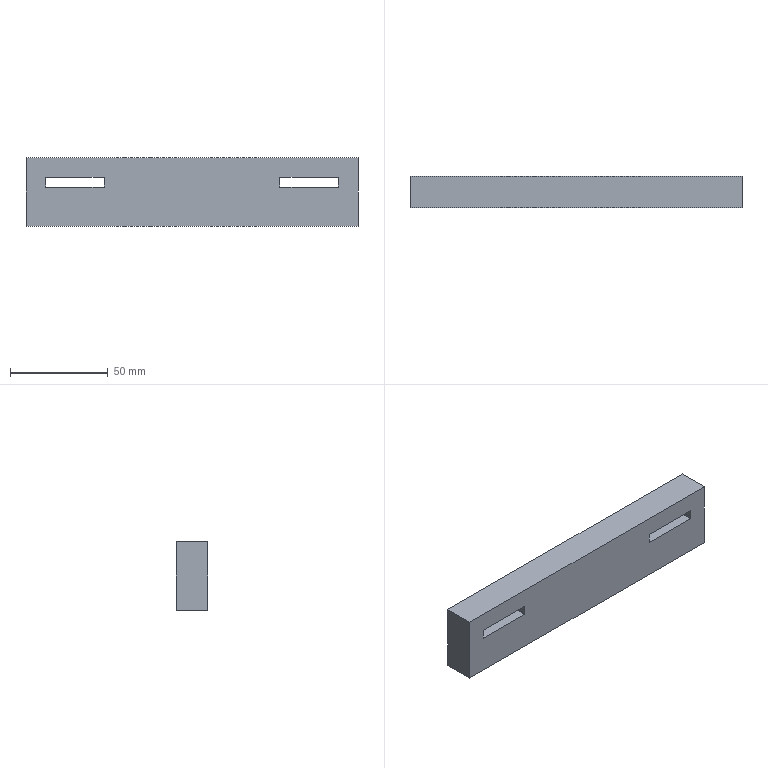Part | STEP file | Tube necking machine_id730_x_t | 1 solid | 14 faces | box 170 x 16 x 35 mm | volume 90400 mm3 | plane 14
STEP:
#1=CARTESIAN_POINT('',(0.,0.,0.));
#2=DIRECTION('',(0.,0.,1.));
#3=DIRECTION('',(1.,0.,0.));
#4=AXIS2_PLACEMENT_3D('',#1,#2,#3);
#5=CARTESIAN_POINT('',(-75.,-243.,191.));
#6=VERTEX_POINT('',#5);
#7=CARTESIAN_POINT('',(-75.,-243.,196.));
#8=VERTEX_POINT('',#7);
#9=CARTESIAN_POINT('',(-75.,-243.,191.));
#10=DIRECTION('',(0.,0.,1.));
#11=VECTOR('',#10,1.);
#12=LINE('',#9,#11);
#13=CARTESIAN_POINT('',(0.,-243.,0.));
#14=DIRECTION('',(0.,-1.,0.));
#15=DIRECTION('',(0.,0.,-1.));
#16=AXIS2_PLACEMENT_3D('',#13,#14,#15);
#17=PLANE('',#16);
#18=CARTESIAN_POINT('',(-191.,-75.));
#19=DIRECTION('',(-1.,0.));
#20=VECTOR('',#19,1.);
#21=LINE('',#18,#20);
#22=(GEOMETRIC_REPRESENTATION_CONTEXT(2)PARAMETRIC_REPRESENTATION_CONTEXT()REPRESENTATION_CONTEXT('',''));
#23=DEFINITIONAL_REPRESENTATION('',(#21),#22);
#24=PCURVE('',#17,#23);
#25=CARTESIAN_POINT('',(-75.,-243.,191.));
#26=DIRECTION('',(1.,0.,0.));
#27=DIRECTION('',(0.,0.,-1.));
#28=AXIS2_PLACEMENT_3D('',#25,#26,#27);
#29=PLANE('',#28);
#30=CARTESIAN_POINT('',(0.,0.));
#31=DIRECTION('',(-1.,0.));
#32=VECTOR('',#31,1.);
#33=LINE('',#30,#32);
#34=(GEOMETRIC_REPRESENTATION_CONTEXT(2)PARAMETRIC_REPRESENTATION_CONTEXT()REPRESENTATION_CONTEXT('',''));
#35=DEFINITIONAL_REPRESENTATION('',(#33),#34);
#36=PCURVE('',#29,#35);
#37=SURFACE_CURVE('',#12,(#24,#36),.PCURVE_S1.);
#38=EDGE_CURVE('',#6,#8,#37,.T.);
#39=ORIENTED_EDGE('',*,*,#38,.F.);
#40=CARTESIAN_POINT('',(-45.,-243.,191.));
#41=VERTEX_POINT('',#40);
#42=CARTESIAN_POINT('',(-40.,-243.,191.));
#43=DIRECTION('',(-1.,0.,0.));
#44=VECTOR('',#43,1.);
#45=LINE('',#42,#44);
#46=CARTESIAN_POINT('',(-191.,-40.));
#47=DIRECTION('',(0.,-1.));
#48=VECTOR('',#47,1.);
#49=LINE('',#46,#48);
#50=(GEOMETRIC_REPRESENTATION_CONTEXT(2)PARAMETRIC_REPRESENTATION_CONTEXT()REPRESENTATION_CONTEXT('',''));
#51=DEFINITIONAL_REPRESENTATION('',(#49),#50);
#52=PCURVE('',#17,#51);
#53=CARTESIAN_POINT('',(-40.,-243.,191.));
#54=DIRECTION('',(0.,0.,1.));
#55=DIRECTION('',(1.,0.,0.));
#56=AXIS2_PLACEMENT_3D('',#53,#54,#55);
#57=PLANE('',#56);
#58=CARTESIAN_POINT('',(0.,0.));
#59=DIRECTION('',(-1.,0.));
#60=VECTOR('',#59,1.);
#61=LINE('',#58,#60);
#62=(GEOMETRIC_REPRESENTATION_CONTEXT(2)PARAMETRIC_REPRESENTATION_CONTEXT()REPRESENTATION_CONTEXT('',''));
#63=DEFINITIONAL_REPRESENTATION('',(#61),#62);
#64=PCURVE('',#57,#63);
#65=SURFACE_CURVE('',#45,(#52,#64),.PCURVE_S1.);
#66=EDGE_CURVE('',#41,#6,#65,.T.);
#67=ORIENTED_EDGE('',*,*,#66,.F.);
#68=CARTESIAN_POINT('',(-45.,-243.,196.));
#69=VERTEX_POINT('',#68);
#70=CARTESIAN_POINT('',(-45.,-243.,0.));
#71=DIRECTION('',(0.,0.,-1.));
#72=VECTOR('',#71,1.);
#73=LINE('',#70,#72);
#74=CARTESIAN_POINT('',(0.,-45.));
#75=DIRECTION('',(1.,0.));
#76=VECTOR('',#75,1.);
#77=LINE('',#74,#76);
#78=(GEOMETRIC_REPRESENTATION_CONTEXT(2)PARAMETRIC_REPRESENTATION_CONTEXT()REPRESENTATION_CONTEXT('',''));
#79=DEFINITIONAL_REPRESENTATION('',(#77),#78);
#80=PCURVE('',#17,#79);
#81=CARTESIAN_POINT('',(-45.,-243.,196.));
#82=DIRECTION('',(-1.,0.,0.));
#83=DIRECTION('',(0.,0.,1.));
#84=AXIS2_PLACEMENT_3D('',#81,#82,#83);
#85=PLANE('',#84);
#86=CARTESIAN_POINT('',(-196.,0.));
#87=DIRECTION('',(-1.,0.));
#88=VECTOR('',#87,1.);
#89=LINE('',#86,#88);
#90=(GEOMETRIC_REPRESENTATION_CONTEXT(2)PARAMETRIC_REPRESENTATION_CONTEXT()REPRESENTATION_CONTEXT('',''));
#91=DEFINITIONAL_REPRESENTATION('',(#89),#90);
#92=PCURVE('',#85,#91);
#93=SURFACE_CURVE('',#73,(#80,#92),.PCURVE_S1.);
#94=EDGE_CURVE('',#69,#41,#93,.T.);
#95=ORIENTED_EDGE('',*,*,#94,.F.);
#96=CARTESIAN_POINT('',(-75.,-243.,196.));
#97=DIRECTION('',(1.,0.,0.));
#98=VECTOR('',#97,1.);
#99=LINE('',#96,#98);
#100=CARTESIAN_POINT('',(-196.,-75.));
#101=DIRECTION('',(0.,1.));
#102=VECTOR('',#101,1.);
#103=LINE('',#100,#102);
#104=(GEOMETRIC_REPRESENTATION_CONTEXT(2)PARAMETRIC_REPRESENTATION_CONTEXT()REPRESENTATION_CONTEXT('',''));
#105=DEFINITIONAL_REPRESENTATION('',(#103),#104);
#106=PCURVE('',#17,#105);
#107=CARTESIAN_POINT('',(-75.,-243.,196.));
#108=DIRECTION('',(0.,0.,-1.));
#109=DIRECTION('',(-1.,0.,0.));
#110=AXIS2_PLACEMENT_3D('',#107,#108,#109);
#111=PLANE('',#110);
#112=CARTESIAN_POINT('',(0.,0.));
#113=DIRECTION('',(-1.,0.));
#114=VECTOR('',#113,1.);
#115=LINE('',#112,#114);
#116=(GEOMETRIC_REPRESENTATION_CONTEXT(2)PARAMETRIC_REPRESENTATION_CONTEXT()REPRESENTATION_CONTEXT('',''));
#117=DEFINITIONAL_REPRESENTATION('',(#115),#116);
#118=PCURVE('',#111,#117);
#119=SURFACE_CURVE('',#99,(#106,#118),.PCURVE_S1.);
#120=EDGE_CURVE('',#8,#69,#119,.T.);
#121=ORIENTED_EDGE('',*,*,#120,.F.);
#122=EDGE_LOOP('',(#39,#67,#95,#121));
#123=FACE_BOUND('',#122,.T.);
#124=CARTESIAN_POINT('',(-85.,-243.,206.));
#125=VERTEX_POINT('',#124);
#126=CARTESIAN_POINT('',(-85.,-243.,171.));
#127=VERTEX_POINT('',#126);
#128=CARTESIAN_POINT('',(-85.,-243.,206.));
#129=DIRECTION('',(0.,0.,-1.));
#130=VECTOR('',#129,1.);
#131=LINE('',#128,#130);
#132=CARTESIAN_POINT('',(-206.,-85.));
#133=DIRECTION('',(1.,0.));
#134=VECTOR('',#133,1.);
#135=LINE('',#132,#134);
#136=(GEOMETRIC_REPRESENTATION_CONTEXT(2)PARAMETRIC_REPRESENTATION_CONTEXT()REPRESENTATION_CONTEXT('',''));
#137=DEFINITIONAL_REPRESENTATION('',(#135),#136);
#138=PCURVE('',#17,#137);
#139=CARTESIAN_POINT('',(-85.,-243.,206.));
#140=DIRECTION('',(-1.,0.,0.));
#141=DIRECTION('',(0.,0.,1.));
#142=AXIS2_PLACEMENT_3D('',#139,#140,#141);
#143=PLANE('',#142);
#144=CARTESIAN_POINT('',(0.,0.));
#145=DIRECTION('',(-1.,0.));
#146=VECTOR('',#145,1.);
#147=LINE('',#144,#146);
#148=(GEOMETRIC_REPRESENTATION_CONTEXT(2)PARAMETRIC_REPRESENTATION_CONTEXT()REPRESENTATION_CONTEXT('',''));
#149=DEFINITIONAL_REPRESENTATION('',(#147),#148);
#150=PCURVE('',#143,#149);
#151=SURFACE_CURVE('',#131,(#138,#150),.PCURVE_S1.);
#152=EDGE_CURVE('',#125,#127,#151,.T.);
#153=ORIENTED_EDGE('',*,*,#152,.F.);
#154=CARTESIAN_POINT('',(85.,-243.,206.));
#155=VERTEX_POINT('',#154);
#156=CARTESIAN_POINT('',(85.,-243.,206.));
#157=DIRECTION('',(-1.,0.,0.));
#158=VECTOR('',#157,1.);
#159=LINE('',#156,#158);
#160=CARTESIAN_POINT('',(-206.,85.));
#161=DIRECTION('',(0.,-1.));
#162=VECTOR('',#161,1.);
#163=LINE('',#160,#162);
#164=(GEOMETRIC_REPRESENTATION_CONTEXT(2)PARAMETRIC_REPRESENTATION_CONTEXT()REPRESENTATION_CONTEXT('',''));
#165=DEFINITIONAL_REPRESENTATION('',(#163),#164);
#166=PCURVE('',#17,#165);
#167=CARTESIAN_POINT('',(85.,-243.,206.));
#168=DIRECTION('',(0.,0.,1.));
#169=DIRECTION('',(1.,0.,0.));
#170=AXIS2_PLACEMENT_3D('',#167,#168,#169);
#171=PLANE('',#170);
#172=CARTESIAN_POINT('',(0.,0.));
#173=DIRECTION('',(-1.,0.));
#174=VECTOR('',#173,1.);
#175=LINE('',#172,#174);
#176=(GEOMETRIC_REPRESENTATION_CONTEXT(2)PARAMETRIC_REPRESENTATION_CONTEXT()REPRESENTATION_CONTEXT('',''));
#177=DEFINITIONAL_REPRESENTATION('',(#175),#176);
#178=PCURVE('',#171,#177);
#179=SURFACE_CURVE('',#159,(#166,#178),.PCURVE_S1.);
#180=EDGE_CURVE('',#155,#125,#179,.T.);
#181=ORIENTED_EDGE('',*,*,#180,.F.);
#182=CARTESIAN_POINT('',(85.,-243.,171.));
#183=VERTEX_POINT('',#182);
#184=CARTESIAN_POINT('',(85.,-243.,171.));
#185=DIRECTION('',(0.,0.,1.));
#186=VECTOR('',#185,1.);
#187=LINE('',#184,#186);
#188=CARTESIAN_POINT('',(-171.,85.));
#189=DIRECTION('',(-1.,0.));
#190=VECTOR('',#189,1.);
#191=LINE('',#188,#190);
#192=(GEOMETRIC_REPRESENTATION_CONTEXT(2)PARAMETRIC_REPRESENTATION_CONTEXT()REPRESENTATION_CONTEXT('',''));
#193=DEFINITIONAL_REPRESENTATION('',(#191),#192);
#194=PCURVE('',#17,#193);
#195=CARTESIAN_POINT('',(85.,-243.,171.));
#196=DIRECTION('',(1.,0.,0.));
#197=DIRECTION('',(0.,0.,-1.));
#198=AXIS2_PLACEMENT_3D('',#195,#196,#197);
#199=PLANE('',#198);
#200=CARTESIAN_POINT('',(0.,0.));
#201=DIRECTION('',(-1.,0.));
#202=VECTOR('',#201,1.);
#203=LINE('',#200,#202);
#204=(GEOMETRIC_REPRESENTATION_CONTEXT(2)PARAMETRIC_REPRESENTATION_CONTEXT()REPRESENTATION_CONTEXT('',''));
#205=DEFINITIONAL_REPRESENTATION('',(#203),#204);
#206=PCURVE('',#199,#205);
#207=SURFACE_CURVE('',#187,(#194,#206),.PCURVE_S1.);
#208=EDGE_CURVE('',#183,#155,#207,.T.);
#209=ORIENTED_EDGE('',*,*,#208,.F.);
#210=CARTESIAN_POINT('',(-85.,-243.,171.));
#211=DIRECTION('',(1.,0.,0.));
#212=VECTOR('',#211,1.);
#213=LINE('',#210,#212);
#214=CARTESIAN_POINT('',(-171.,-85.));
#215=DIRECTION('',(0.,1.));
#216=VECTOR('',#215,1.);
#217=LINE('',#214,#216);
#218=(GEOMETRIC_REPRESENTATION_CONTEXT(2)PARAMETRIC_REPRESENTATION_CONTEXT()REPRESENTATION_CONTEXT('',''));
#219=DEFINITIONAL_REPRESENTATION('',(#217),#218);
#220=PCURVE('',#17,#219);
#221=CARTESIAN_POINT('',(-85.,-243.,171.));
#222=DIRECTION('',(0.,0.,-1.));
#223=DIRECTION('',(-1.,0.,0.));
#224=AXIS2_PLACEMENT_3D('',#221,#222,#223);
#225=PLANE('',#224);
#226=CARTESIAN_POINT('',(0.,0.));
#227=DIRECTION('',(-1.,0.));
#228=VECTOR('',#227,1.);
#229=LINE('',#226,#228);
#230=(GEOMETRIC_REPRESENTATION_CONTEXT(2)PARAMETRIC_REPRESENTATION_CONTEXT()REPRESENTATION_CONTEXT('',''));
#231=DEFINITIONAL_REPRESENTATION('',(#229),#230);
#232=PCURVE('',#225,#231);
#233=SURFACE_CURVE('',#213,(#220,#232),.PCURVE_S1.);
#234=EDGE_CURVE('',#127,#183,#233,.T.);
#235=ORIENTED_EDGE('',*,*,#234,.F.);
#236=EDGE_LOOP('',(#153,#181,#209,#235));
#237=FACE_BOUND('',#236,.T.);
#238=CARTESIAN_POINT('',(45.,-243.,196.));
#239=VERTEX_POINT('',#238);
#240=CARTESIAN_POINT('',(75.,-243.,196.));
#241=VERTEX_POINT('',#240);
#242=CARTESIAN_POINT('',(0.,-243.,196.));
#243=DIRECTION('',(1.,0.,0.));
#244=VECTOR('',#243,1.);
#245=LINE('',#242,#244);
#246=CARTESIAN_POINT('',(-196.,0.));
#247=DIRECTION('',(0.,1.));
#248=VECTOR('',#247,1.);
#249=LINE('',#246,#248);
#250=(GEOMETRIC_REPRESENTATION_CONTEXT(2)PARAMETRIC_REPRESENTATION_CONTEXT()REPRESENTATION_CONTEXT('',''));
#251=DEFINITIONAL_REPRESENTATION('',(#249),#250);
#252=PCURVE('',#17,#251);
#253=CARTESIAN_POINT('',(40.,-259.,196.));
#254=DIRECTION('',(0.,0.,-1.));
#255=DIRECTION('',(1.,0.,0.));
#256=AXIS2_PLACEMENT_3D('',#253,#254,#255);
#257=PLANE('',#256);
#258=CARTESIAN_POINT('',(-40.,-16.));
#259=DIRECTION('',(1.,0.));
#260=VECTOR('',#259,1.);
#261=LINE('',#258,#260);
#262=(GEOMETRIC_REPRESENTATION_CONTEXT(2)PARAMETRIC_REPRESENTATION_CONTEXT()REPRESENTATION_CONTEXT('',''));
#263=DEFINITIONAL_REPRESENTATION('',(#261),#262);
#264=PCURVE('',#257,#263);
#265=SURFACE_CURVE('',#245,(#252,#264),.PCURVE_S1.);
#266=EDGE_CURVE('',#239,#241,#265,.T.);
#267=ORIENTED_EDGE('',*,*,#266,.F.);
#268=CARTESIAN_POINT('',(45.,-243.,191.));
#269=VERTEX_POINT('',#268);
#270=CARTESIAN_POINT('',(45.,-243.,0.));
#271=DIRECTION('',(0.,0.,1.));
#272=VECTOR('',#271,1.);
#273=LINE('',#270,#272);
#274=CARTESIAN_POINT('',(0.,45.));
#275=DIRECTION('',(-1.,0.));
#276=VECTOR('',#275,1.);
#277=LINE('',#274,#276);
#278=(GEOMETRIC_REPRESENTATION_CONTEXT(2)PARAMETRIC_REPRESENTATION_CONTEXT()REPRESENTATION_CONTEXT('',''));
#279=DEFINITIONAL_REPRESENTATION('',(#277),#278);
#280=PCURVE('',#17,#279);
#281=CARTESIAN_POINT('',(45.,-259.,191.));
#282=DIRECTION('',(1.,0.,0.));
#283=DIRECTION('',(0.,0.,1.));
#284=AXIS2_PLACEMENT_3D('',#281,#282,#283);
#285=PLANE('',#284);
#286=CARTESIAN_POINT('',(-191.,-16.));
#287=DIRECTION('',(1.,0.));
#288=VECTOR('',#287,1.);
#289=LINE('',#286,#288);
#290=(GEOMETRIC_REPRESENTATION_CONTEXT(2)PARAMETRIC_REPRESENTATION_CONTEXT()REPRESENTATION_CONTEXT('',''));
#291=DEFINITIONAL_REPRESENTATION('',(#289),#290);
#292=PCURVE('',#285,#291);
#293=SURFACE_CURVE('',#273,(#280,#292),.PCURVE_S1.);
#294=EDGE_CURVE('',#269,#239,#293,.T.);
#295=ORIENTED_EDGE('',*,*,#294,.F.);
#296=CARTESIAN_POINT('',(75.,-243.,191.));
#297=VERTEX_POINT('',#296);
#298=CARTESIAN_POINT('',(0.,-243.,191.));
#299=DIRECTION('',(-1.,0.,0.));
#300=VECTOR('',#299,1.);
#301=LINE('',#298,#300);
#302=CARTESIAN_POINT('',(-191.,0.));
#303=DIRECTION('',(0.,-1.));
#304=VECTOR('',#303,1.);
#305=LINE('',#302,#304);
#306=(GEOMETRIC_REPRESENTATION_CONTEXT(2)PARAMETRIC_REPRESENTATION_CONTEXT()REPRESENTATION_CONTEXT('',''));
#307=DEFINITIONAL_REPRESENTATION('',(#305),#306);
#308=PCURVE('',#17,#307);
#309=CARTESIAN_POINT('',(75.,-259.,191.));
#310=DIRECTION('',(0.,0.,1.));
#311=DIRECTION('',(-1.,0.,0.));
#312=AXIS2_PLACEMENT_3D('',#309,#310,#311);
#313=PLANE('',#312);
#314=CARTESIAN_POINT('',(75.,-16.));
#315=DIRECTION('',(1.,0.));
#316=VECTOR('',#315,1.);
#317=LINE('',#314,#316);
#318=(GEOMETRIC_REPRESENTATION_CONTEXT(2)PARAMETRIC_REPRESENTATION_CONTEXT()REPRESENTATION_CONTEXT('',''));
#319=DEFINITIONAL_REPRESENTATION('',(#317),#318);
#320=PCURVE('',#313,#319);
#321=SURFACE_CURVE('',#301,(#308,#320),.PCURVE_S1.);
#322=EDGE_CURVE('',#297,#269,#321,.T.);
#323=ORIENTED_EDGE('',*,*,#322,.F.);
#324=CARTESIAN_POINT('',(75.,-243.,0.));
#325=DIRECTION('',(0.,0.,-1.));
#326=VECTOR('',#325,1.);
#327=LINE('',#324,#326);
#328=CARTESIAN_POINT('',(0.,75.));
#329=DIRECTION('',(1.,0.));
#330=VECTOR('',#329,1.);
#331=LINE('',#328,#330);
#332=(GEOMETRIC_REPRESENTATION_CONTEXT(2)PARAMETRIC_REPRESENTATION_CONTEXT()REPRESENTATION_CONTEXT('',''));
#333=DEFINITIONAL_REPRESENTATION('',(#331),#332);
#334=PCURVE('',#17,#333);
#335=CARTESIAN_POINT('',(75.,-259.,196.));
#336=DIRECTION('',(-1.,0.,0.));
#337=DIRECTION('',(0.,0.,-1.));
#338=AXIS2_PLACEMENT_3D('',#335,#336,#337);
#339=PLANE('',#338);
#340=CARTESIAN_POINT('',(196.,-16.));
#341=DIRECTION('',(1.,0.));
#342=VECTOR('',#341,1.);
#343=LINE('',#340,#342);
#344=(GEOMETRIC_REPRESENTATION_CONTEXT(2)PARAMETRIC_REPRESENTATION_CONTEXT()REPRESENTATION_CONTEXT('',''));
#345=DEFINITIONAL_REPRESENTATION('',(#343),#344);
#346=PCURVE('',#339,#345);
#347=SURFACE_CURVE('',#327,(#334,#346),.PCURVE_S1.);
#348=EDGE_CURVE('',#241,#297,#347,.T.);
#349=ORIENTED_EDGE('',*,*,#348,.F.);
#350=EDGE_LOOP('',(#267,#295,#323,#349));
#351=FACE_BOUND('',#350,.T.);
#352=ADVANCED_FACE('',(#123,#237,#351),#17,.F.);
#353=CARTESIAN_POINT('',(-85.,-259.,206.));
#354=VERTEX_POINT('',#353);
#355=CARTESIAN_POINT('',(-85.,-259.,171.));
#356=VERTEX_POINT('',#355);
#357=CARTESIAN_POINT('',(-85.,-259.,206.));
#358=DIRECTION('',(0.,0.,-1.));
#359=VECTOR('',#358,1.);
#360=LINE('',#357,#359);
#361=CARTESIAN_POINT('',(0.,-259.,0.));
#362=DIRECTION('',(0.,-1.,0.));
#363=DIRECTION('',(0.,0.,-1.));
#364=AXIS2_PLACEMENT_3D('',#361,#362,#363);
#365=PLANE('',#364);
#366=CARTESIAN_POINT('',(-206.,-85.));
#367=DIRECTION('',(1.,0.));
#368=VECTOR('',#367,1.);
#369=LINE('',#366,#368);
#370=(GEOMETRIC_REPRESENTATION_CONTEXT(2)PARAMETRIC_REPRESENTATION_CONTEXT()REPRESENTATION_CONTEXT('',''));
#371=DEFINITIONAL_REPRESENTATION('',(#369),#370);
#372=PCURVE('',#365,#371);
#373=CARTESIAN_POINT('',(0.,-16.));
#374=DIRECTION('',(-1.,0.));
#375=VECTOR('',#374,1.);
#376=LINE('',#373,#375);
#377=(GEOMETRIC_REPRESENTATION_CONTEXT(2)PARAMETRIC_REPRESENTATION_CONTEXT()REPRESENTATION_CONTEXT('',''));
#378=DEFINITIONAL_REPRESENTATION('',(#376),#377);
#379=PCURVE('',#143,#378);
#380=SURFACE_CURVE('',#360,(#372,#379),.PCURVE_S1.);
#381=EDGE_CURVE('',#354,#356,#380,.T.);
#382=ORIENTED_EDGE('',*,*,#381,.T.);
#383=CARTESIAN_POINT('',(85.,-259.,171.));
#384=VERTEX_POINT('',#383);
#385=CARTESIAN_POINT('',(-85.,-259.,171.));
#386=DIRECTION('',(1.,0.,0.));
#387=VECTOR('',#386,1.);
#388=LINE('',#385,#387);
#389=CARTESIAN_POINT('',(-171.,-85.));
#390=DIRECTION('',(0.,1.));
#391=VECTOR('',#390,1.);
#392=LINE('',#389,#391);
#393=(GEOMETRIC_REPRESENTATION_CONTEXT(2)PARAMETRIC_REPRESENTATION_CONTEXT()REPRESENTATION_CONTEXT('',''));
#394=DEFINITIONAL_REPRESENTATION('',(#392),#393);
#395=PCURVE('',#365,#394);
#396=CARTESIAN_POINT('',(0.,-16.));
#397=DIRECTION('',(-1.,0.));
#398=VECTOR('',#397,1.);
#399=LINE('',#396,#398);
#400=(GEOMETRIC_REPRESENTATION_CONTEXT(2)PARAMETRIC_REPRESENTATION_CONTEXT()REPRESENTATION_CONTEXT('',''));
#401=DEFINITIONAL_REPRESENTATION('',(#399),#400);
#402=PCURVE('',#225,#401);
#403=SURFACE_CURVE('',#388,(#395,#402),.PCURVE_S1.);
#404=EDGE_CURVE('',#356,#384,#403,.T.);
#405=ORIENTED_EDGE('',*,*,#404,.T.);
#406=CARTESIAN_POINT('',(85.,-259.,206.));
#407=VERTEX_POINT('',#406);
#408=CARTESIAN_POINT('',(85.,-259.,171.));
#409=DIRECTION('',(0.,0.,1.));
#410=VECTOR('',#409,1.);
#411=LINE('',#408,#410);
#412=CARTESIAN_POINT('',(-171.,85.));
#413=DIRECTION('',(-1.,0.));
#414=VECTOR('',#413,1.);
#415=LINE('',#412,#414);
#416=(GEOMETRIC_REPRESENTATION_CONTEXT(2)PARAMETRIC_REPRESENTATION_CONTEXT()REPRESENTATION_CONTEXT('',''));
#417=DEFINITIONAL_REPRESENTATION('',(#415),#416);
#418=PCURVE('',#365,#417);
#419=CARTESIAN_POINT('',(0.,-16.));
#420=DIRECTION('',(-1.,0.));
#421=VECTOR('',#420,1.);
#422=LINE('',#419,#421);
#423=(GEOMETRIC_REPRESENTATION_CONTEXT(2)PARAMETRIC_REPRESENTATION_CONTEXT()REPRESENTATION_CONTEXT('',''));
#424=DEFINITIONAL_REPRESENTATION('',(#422),#423);
#425=PCURVE('',#199,#424);
#426=SURFACE_CURVE('',#411,(#418,#425),.PCURVE_S1.);
#427=EDGE_CURVE('',#384,#407,#426,.T.);
#428=ORIENTED_EDGE('',*,*,#427,.T.);
#429=CARTESIAN_POINT('',(85.,-259.,206.));
#430=DIRECTION('',(-1.,0.,0.));
#431=VECTOR('',#430,1.);
#432=LINE('',#429,#431);
#433=CARTESIAN_POINT('',(-206.,85.));
#434=DIRECTION('',(0.,-1.));
#435=VECTOR('',#434,1.);
#436=LINE('',#433,#435);
#437=(GEOMETRIC_REPRESENTATION_CONTEXT(2)PARAMETRIC_REPRESENTATION_CONTEXT()REPRESENTATION_CONTEXT('',''));
#438=DEFINITIONAL_REPRESENTATION('',(#436),#437);
#439=PCURVE('',#365,#438);
#440=CARTESIAN_POINT('',(0.,-16.));
#441=DIRECTION('',(-1.,0.));
#442=VECTOR('',#441,1.);
#443=LINE('',#440,#442);
#444=(GEOMETRIC_REPRESENTATION_CONTEXT(2)PARAMETRIC_REPRESENTATION_CONTEXT()REPRESENTATION_CONTEXT('',''));
#445=DEFINITIONAL_REPRESENTATION('',(#443),#444);
#446=PCURVE('',#171,#445);
#447=SURFACE_CURVE('',#432,(#439,#446),.PCURVE_S1.);
#448=EDGE_CURVE('',#407,#354,#447,.T.);
#449=ORIENTED_EDGE('',*,*,#448,.T.);
#450=EDGE_LOOP('',(#382,#405,#428,#449));
#451=FACE_BOUND('',#450,.T.);
#452=CARTESIAN_POINT('',(-75.,-259.,191.));
#453=VERTEX_POINT('',#452);
#454=CARTESIAN_POINT('',(-75.,-259.,196.));
#455=VERTEX_POINT('',#454);
#456=CARTESIAN_POINT('',(-75.,-259.,191.));
#457=DIRECTION('',(0.,0.,1.));
#458=VECTOR('',#457,1.);
#459=LINE('',#456,#458);
#460=CARTESIAN_POINT('',(-191.,-75.));
#461=DIRECTION('',(-1.,0.));
#462=VECTOR('',#461,1.);
#463=LINE('',#460,#462);
#464=(GEOMETRIC_REPRESENTATION_CONTEXT(2)PARAMETRIC_REPRESENTATION_CONTEXT()REPRESENTATION_CONTEXT('',''));
#465=DEFINITIONAL_REPRESENTATION('',(#463),#464);
#466=PCURVE('',#365,#465);
#467=CARTESIAN_POINT('',(0.,-16.));
#468=DIRECTION('',(-1.,0.));
#469=VECTOR('',#468,1.);
#470=LINE('',#467,#469);
#471=(GEOMETRIC_REPRESENTATION_CONTEXT(2)PARAMETRIC_REPRESENTATION_CONTEXT()REPRESENTATION_CONTEXT('',''));
#472=DEFINITIONAL_REPRESENTATION('',(#470),#471);
#473=PCURVE('',#29,#472);
#474=SURFACE_CURVE('',#459,(#466,#473),.PCURVE_S1.);
#475=EDGE_CURVE('',#453,#455,#474,.T.);
#476=ORIENTED_EDGE('',*,*,#475,.T.);
#477=CARTESIAN_POINT('',(-45.,-259.,196.));
#478=VERTEX_POINT('',#477);
#479=CARTESIAN_POINT('',(-75.,-259.,196.));
#480=DIRECTION('',(1.,0.,0.));
#481=VECTOR('',#480,1.);
#482=LINE('',#479,#481);
#483=CARTESIAN_POINT('',(-196.,-75.));
#484=DIRECTION('',(0.,1.));
#485=VECTOR('',#484,1.);
#486=LINE('',#483,#485);
#487=(GEOMETRIC_REPRESENTATION_CONTEXT(2)PARAMETRIC_REPRESENTATION_CONTEXT()REPRESENTATION_CONTEXT('',''));
#488=DEFINITIONAL_REPRESENTATION('',(#486),#487);
#489=PCURVE('',#365,#488);
#490=CARTESIAN_POINT('',(0.,-16.));
#491=DIRECTION('',(-1.,0.));
#492=VECTOR('',#491,1.);
#493=LINE('',#490,#492);
#494=(GEOMETRIC_REPRESENTATION_CONTEXT(2)PARAMETRIC_REPRESENTATION_CONTEXT()REPRESENTATION_CONTEXT('',''));
#495=DEFINITIONAL_REPRESENTATION('',(#493),#494);
#496=PCURVE('',#111,#495);
#497=SURFACE_CURVE('',#482,(#489,#496),.PCURVE_S1.);
#498=EDGE_CURVE('',#455,#478,#497,.T.);
#499=ORIENTED_EDGE('',*,*,#498,.T.);
#500=CARTESIAN_POINT('',(-45.,-259.,191.));
#501=VERTEX_POINT('',#500);
#502=CARTESIAN_POINT('',(-45.,-259.,0.));
#503=DIRECTION('',(0.,0.,-1.));
#504=VECTOR('',#503,1.);
#505=LINE('',#502,#504);
#506=CARTESIAN_POINT('',(0.,-45.));
#507=DIRECTION('',(1.,0.));
#508=VECTOR('',#507,1.);
#509=LINE('',#506,#508);
#510=(GEOMETRIC_REPRESENTATION_CONTEXT(2)PARAMETRIC_REPRESENTATION_CONTEXT()REPRESENTATION_CONTEXT('',''));
#511=DEFINITIONAL_REPRESENTATION('',(#509),#510);
#512=PCURVE('',#365,#511);
#513=CARTESIAN_POINT('',(-196.,-16.));
#514=DIRECTION('',(-1.,0.));
#515=VECTOR('',#514,1.);
#516=LINE('',#513,#515);
#517=(GEOMETRIC_REPRESENTATION_CONTEXT(2)PARAMETRIC_REPRESENTATION_CONTEXT()REPRESENTATION_CONTEXT('',''));
#518=DEFINITIONAL_REPRESENTATION('',(#516),#517);
#519=PCURVE('',#85,#518);
#520=SURFACE_CURVE('',#505,(#512,#519),.PCURVE_S1.);
#521=EDGE_CURVE('',#478,#501,#520,.T.);
#522=ORIENTED_EDGE('',*,*,#521,.T.);
#523=CARTESIAN_POINT('',(-40.,-259.,191.));
#524=DIRECTION('',(-1.,0.,0.));
#525=VECTOR('',#524,1.);
#526=LINE('',#523,#525);
#527=CARTESIAN_POINT('',(-191.,-40.));
#528=DIRECTION('',(0.,-1.));
#529=VECTOR('',#528,1.);
#530=LINE('',#527,#529);
#531=(GEOMETRIC_REPRESENTATION_CONTEXT(2)PARAMETRIC_REPRESENTATION_CONTEXT()REPRESENTATION_CONTEXT('',''));
#532=DEFINITIONAL_REPRESENTATION('',(#530),#531);
#533=PCURVE('',#365,#532);
#534=CARTESIAN_POINT('',(0.,-16.));
#535=DIRECTION('',(-1.,0.));
#536=VECTOR('',#535,1.);
#537=LINE('',#534,#536);
#538=(GEOMETRIC_REPRESENTATION_CONTEXT(2)PARAMETRIC_REPRESENTATION_CONTEXT()REPRESENTATION_CONTEXT('',''));
#539=DEFINITIONAL_REPRESENTATION('',(#537),#538);
#540=PCURVE('',#57,#539);
#541=SURFACE_CURVE('',#526,(#533,#540),.PCURVE_S1.);
#542=EDGE_CURVE('',#501,#453,#541,.T.);
#543=ORIENTED_EDGE('',*,*,#542,.T.);
#544=EDGE_LOOP('',(#476,#499,#522,#543));
#545=FACE_BOUND('',#544,.T.);
#546=CARTESIAN_POINT('',(45.,-259.,196.));
#547=VERTEX_POINT('',#546);
#548=CARTESIAN_POINT('',(45.,-259.,191.));
#549=VERTEX_POINT('',#548);
#550=CARTESIAN_POINT('',(45.,-259.,191.));
#551=DIRECTION('',(0.,0.,-1.));
#552=VECTOR('',#551,1.);
#553=LINE('',#550,#552);
#554=CARTESIAN_POINT('',(-191.,45.));
#555=DIRECTION('',(1.,0.));
#556=VECTOR('',#555,1.);
#557=LINE('',#554,#556);
#558=(GEOMETRIC_REPRESENTATION_CONTEXT(2)PARAMETRIC_REPRESENTATION_CONTEXT()REPRESENTATION_CONTEXT('',''));
#559=DEFINITIONAL_REPRESENTATION('',(#557),#558);
#560=PCURVE('',#365,#559);
#561=CARTESIAN_POINT('',(0.,0.));
#562=DIRECTION('',(-1.,0.));
#563=VECTOR('',#562,1.);
#564=LINE('',#561,#563);
#565=(GEOMETRIC_REPRESENTATION_CONTEXT(2)PARAMETRIC_REPRESENTATION_CONTEXT()REPRESENTATION_CONTEXT('',''));
#566=DEFINITIONAL_REPRESENTATION('',(#564),#565);
#567=PCURVE('',#285,#566);
#568=SURFACE_CURVE('',#553,(#560,#567),.PCURVE_S1.);
#569=EDGE_CURVE('',#547,#549,#568,.T.);
#570=ORIENTED_EDGE('',*,*,#569,.F.);
#571=CARTESIAN_POINT('',(75.,-259.,196.));
#572=VERTEX_POINT('',#571);
#573=CARTESIAN_POINT('',(40.,-259.,196.));
#574=DIRECTION('',(-1.,0.,0.));
#575=VECTOR('',#574,1.);
#576=LINE('',#573,#575);
#577=CARTESIAN_POINT('',(-196.,40.));
#578=DIRECTION('',(0.,-1.));
#579=VECTOR('',#578,1.);
#580=LINE('',#577,#579);
#581=(GEOMETRIC_REPRESENTATION_CONTEXT(2)PARAMETRIC_REPRESENTATION_CONTEXT()REPRESENTATION_CONTEXT('',''));
#582=DEFINITIONAL_REPRESENTATION('',(#580),#581);
#583=PCURVE('',#365,#582);
#584=CARTESIAN_POINT('',(0.,0.));
#585=DIRECTION('',(-1.,0.));
#586=VECTOR('',#585,1.);
#587=LINE('',#584,#586);
#588=(GEOMETRIC_REPRESENTATION_CONTEXT(2)PARAMETRIC_REPRESENTATION_CONTEXT()REPRESENTATION_CONTEXT('',''));
#589=DEFINITIONAL_REPRESENTATION('',(#587),#588);
#590=PCURVE('',#257,#589);
#591=SURFACE_CURVE('',#576,(#583,#590),.PCURVE_S1.);
#592=EDGE_CURVE('',#572,#547,#591,.T.);
#593=ORIENTED_EDGE('',*,*,#592,.F.);
#594=CARTESIAN_POINT('',(75.,-259.,191.));
#595=VERTEX_POINT('',#594);
#596=CARTESIAN_POINT('',(75.,-259.,196.));
#597=DIRECTION('',(0.,0.,1.));
#598=VECTOR('',#597,1.);
#599=LINE('',#596,#598);
#600=CARTESIAN_POINT('',(-196.,75.));
#601=DIRECTION('',(-1.,0.));
#602=VECTOR('',#601,1.);
#603=LINE('',#600,#602);
#604=(GEOMETRIC_REPRESENTATION_CONTEXT(2)PARAMETRIC_REPRESENTATION_CONTEXT()REPRESENTATION_CONTEXT('',''));
#605=DEFINITIONAL_REPRESENTATION('',(#603),#604);
#606=PCURVE('',#365,#605);
#607=CARTESIAN_POINT('',(0.,0.));
#608=DIRECTION('',(-1.,0.));
#609=VECTOR('',#608,1.);
#610=LINE('',#607,#609);
#611=(GEOMETRIC_REPRESENTATION_CONTEXT(2)PARAMETRIC_REPRESENTATION_CONTEXT()REPRESENTATION_CONTEXT('',''));
#612=DEFINITIONAL_REPRESENTATION('',(#610),#611);
#613=PCURVE('',#339,#612);
#614=SURFACE_CURVE('',#599,(#606,#613),.PCURVE_S1.);
#615=EDGE_CURVE('',#595,#572,#614,.T.);
#616=ORIENTED_EDGE('',*,*,#615,.F.);
#617=CARTESIAN_POINT('',(75.,-259.,191.));
#618=DIRECTION('',(1.,0.,0.));
#619=VECTOR('',#618,1.);
#620=LINE('',#617,#619);
#621=CARTESIAN_POINT('',(-191.,75.));
#622=DIRECTION('',(0.,1.));
#623=VECTOR('',#622,1.);
#624=LINE('',#621,#623);
#625=(GEOMETRIC_REPRESENTATION_CONTEXT(2)PARAMETRIC_REPRESENTATION_CONTEXT()REPRESENTATION_CONTEXT('',''));
#626=DEFINITIONAL_REPRESENTATION('',(#624),#625);
#627=PCURVE('',#365,#626);
#628=CARTESIAN_POINT('',(0.,0.));
#629=DIRECTION('',(-1.,0.));
#630=VECTOR('',#629,1.);
#631=LINE('',#628,#630);
#632=(GEOMETRIC_REPRESENTATION_CONTEXT(2)PARAMETRIC_REPRESENTATION_CONTEXT()REPRESENTATION_CONTEXT('',''));
#633=DEFINITIONAL_REPRESENTATION('',(#631),#632);
#634=PCURVE('',#313,#633);
#635=SURFACE_CURVE('',#620,(#627,#634),.PCURVE_S1.);
#636=EDGE_CURVE('',#549,#595,#635,.T.);
#637=ORIENTED_EDGE('',*,*,#636,.F.);
#638=EDGE_LOOP('',(#570,#593,#616,#637));
#639=FACE_BOUND('',#638,.T.);
#640=ADVANCED_FACE('',(#451,#545,#639),#365,.T.);
#641=ORIENTED_EDGE('',*,*,#475,.F.);
#642=CARTESIAN_POINT('',(-75.,-243.,191.));
#643=DIRECTION('',(0.,-1.,0.));
#644=VECTOR('',#643,1.);
#645=LINE('',#642,#644);
#646=CARTESIAN_POINT('',(0.,0.));
#647=DIRECTION('',(0.,-1.));
#648=VECTOR('',#647,1.);
#649=LINE('',#646,#648);
#650=(GEOMETRIC_REPRESENTATION_CONTEXT(2)PARAMETRIC_REPRESENTATION_CONTEXT()REPRESENTATION_CONTEXT('',''));
#651=DEFINITIONAL_REPRESENTATION('',(#649),#650);
#652=PCURVE('',#29,#651);
#653=CARTESIAN_POINT('',(-35.,0.));
#654=DIRECTION('',(0.,-1.));
#655=VECTOR('',#654,1.);
#656=LINE('',#653,#655);
#657=(GEOMETRIC_REPRESENTATION_CONTEXT(2)PARAMETRIC_REPRESENTATION_CONTEXT()REPRESENTATION_CONTEXT('',''));
#658=DEFINITIONAL_REPRESENTATION('',(#656),#657);
#659=PCURVE('',#57,#658);
#660=SURFACE_CURVE('',#645,(#652,#659),.PCURVE_S1.);
#661=EDGE_CURVE('',#6,#453,#660,.T.);
#662=ORIENTED_EDGE('',*,*,#661,.F.);
#663=ORIENTED_EDGE('',*,*,#38,.T.);
#664=CARTESIAN_POINT('',(-75.,-243.,196.));
#665=DIRECTION('',(0.,-1.,0.));
#666=VECTOR('',#665,1.);
#667=LINE('',#664,#666);
#668=CARTESIAN_POINT('',(-5.,0.));
#669=DIRECTION('',(0.,-1.));
#670=VECTOR('',#669,1.);
#671=LINE('',#668,#670);
#672=(GEOMETRIC_REPRESENTATION_CONTEXT(2)PARAMETRIC_REPRESENTATION_CONTEXT()REPRESENTATION_CONTEXT('',''));
#673=DEFINITIONAL_REPRESENTATION('',(#671),#672);
#674=PCURVE('',#29,#673);
#675=CARTESIAN_POINT('',(0.,0.));
#676=DIRECTION('',(0.,-1.));
#677=VECTOR('',#676,1.);
#678=LINE('',#675,#677);
#679=(GEOMETRIC_REPRESENTATION_CONTEXT(2)PARAMETRIC_REPRESENTATION_CONTEXT()REPRESENTATION_CONTEXT('',''));
#680=DEFINITIONAL_REPRESENTATION('',(#678),#679);
#681=PCURVE('',#111,#680);
#682=SURFACE_CURVE('',#667,(#674,#681),.PCURVE_S1.);
#683=EDGE_CURVE('',#8,#455,#682,.T.);
#684=ORIENTED_EDGE('',*,*,#683,.T.);
#685=EDGE_LOOP('',(#641,#662,#663,#684));
#686=FACE_BOUND('',#685,.T.);
#687=ADVANCED_FACE('',(#686),#29,.T.);
#688=ORIENTED_EDGE('',*,*,#498,.F.);
#689=ORIENTED_EDGE('',*,*,#683,.F.);
#690=ORIENTED_EDGE('',*,*,#120,.T.);
#691=CARTESIAN_POINT('',(-45.,-243.,196.));
#692=DIRECTION('',(0.,-1.,0.));
#693=VECTOR('',#692,1.);
#694=LINE('',#691,#693);
#695=CARTESIAN_POINT('',(-30.,0.));
#696=DIRECTION('',(0.,-1.));
#697=VECTOR('',#696,1.);
#698=LINE('',#695,#697);
#699=(GEOMETRIC_REPRESENTATION_CONTEXT(2)PARAMETRIC_REPRESENTATION_CONTEXT()REPRESENTATION_CONTEXT('',''));
#700=DEFINITIONAL_REPRESENTATION('',(#698),#699);
#701=PCURVE('',#111,#700);
#702=CARTESIAN_POINT('',(0.,0.));
#703=DIRECTION('',(0.,-1.));
#704=VECTOR('',#703,1.);
#705=LINE('',#702,#704);
#706=(GEOMETRIC_REPRESENTATION_CONTEXT(2)PARAMETRIC_REPRESENTATION_CONTEXT()REPRESENTATION_CONTEXT('',''));
#707=DEFINITIONAL_REPRESENTATION('',(#705),#706);
#708=PCURVE('',#85,#707);
#709=SURFACE_CURVE('',#694,(#701,#708),.PCURVE_S1.);
#710=EDGE_CURVE('',#69,#478,#709,.T.);
#711=ORIENTED_EDGE('',*,*,#710,.T.);
#712=EDGE_LOOP('',(#688,#689,#690,#711));
#713=FACE_BOUND('',#712,.T.);
#714=ADVANCED_FACE('',(#713),#111,.T.);
#715=ORIENTED_EDGE('',*,*,#521,.F.);
#716=ORIENTED_EDGE('',*,*,#710,.F.);
#717=ORIENTED_EDGE('',*,*,#94,.T.);
#718=CARTESIAN_POINT('',(-45.,-243.,191.));
#719=DIRECTION('',(0.,-1.,0.));
#720=VECTOR('',#719,1.);
#721=LINE('',#718,#720);
#722=CARTESIAN_POINT('',(-5.,0.));
#723=DIRECTION('',(0.,-1.));
#724=VECTOR('',#723,1.);
#725=LINE('',#722,#724);
#726=(GEOMETRIC_REPRESENTATION_CONTEXT(2)PARAMETRIC_REPRESENTATION_CONTEXT()REPRESENTATION_CONTEXT('',''));
#727=DEFINITIONAL_REPRESENTATION('',(#725),#726);
#728=PCURVE('',#85,#727);
#729=CARTESIAN_POINT('',(-5.,0.));
#730=DIRECTION('',(0.,-1.));
#731=VECTOR('',#730,1.);
#732=LINE('',#729,#731);
#733=(GEOMETRIC_REPRESENTATION_CONTEXT(2)PARAMETRIC_REPRESENTATION_CONTEXT()REPRESENTATION_CONTEXT('',''));
#734=DEFINITIONAL_REPRESENTATION('',(#732),#733);
#735=PCURVE('',#57,#734);
#736=SURFACE_CURVE('',#721,(#728,#735),.PCURVE_S1.);
#737=EDGE_CURVE('',#41,#501,#736,.T.);
#738=ORIENTED_EDGE('',*,*,#737,.T.);
#739=EDGE_LOOP('',(#715,#716,#717,#738));
#740=FACE_BOUND('',#739,.T.);
#741=ADVANCED_FACE('',(#740),#85,.T.);
#742=ORIENTED_EDGE('',*,*,#381,.F.);
#743=CARTESIAN_POINT('',(-85.,-243.,206.));
#744=DIRECTION('',(0.,-1.,0.));
#745=VECTOR('',#744,1.);
#746=LINE('',#743,#745);
#747=CARTESIAN_POINT('',(0.,0.));
#748=DIRECTION('',(0.,-1.));
#749=VECTOR('',#748,1.);
#750=LINE('',#747,#749);
#751=(GEOMETRIC_REPRESENTATION_CONTEXT(2)PARAMETRIC_REPRESENTATION_CONTEXT()REPRESENTATION_CONTEXT('',''));
#752=DEFINITIONAL_REPRESENTATION('',(#750),#751);
#753=PCURVE('',#143,#752);
#754=CARTESIAN_POINT('',(-170.,0.));
#755=DIRECTION('',(0.,-1.));
#756=VECTOR('',#755,1.);
#757=LINE('',#754,#756);
#758=(GEOMETRIC_REPRESENTATION_CONTEXT(2)PARAMETRIC_REPRESENTATION_CONTEXT()REPRESENTATION_CONTEXT('',''));
#759=DEFINITIONAL_REPRESENTATION('',(#757),#758);
#760=PCURVE('',#171,#759);
#761=SURFACE_CURVE('',#746,(#753,#760),.PCURVE_S1.);
#762=EDGE_CURVE('',#125,#354,#761,.T.);
#763=ORIENTED_EDGE('',*,*,#762,.F.);
#764=ORIENTED_EDGE('',*,*,#152,.T.);
#765=CARTESIAN_POINT('',(-85.,-243.,171.));
#766=DIRECTION('',(0.,-1.,0.));
#767=VECTOR('',#766,1.);
#768=LINE('',#765,#767);
#769=CARTESIAN_POINT('',(-35.,0.));
#770=DIRECTION('',(0.,-1.));
#771=VECTOR('',#770,1.);
#772=LINE('',#769,#771);
#773=(GEOMETRIC_REPRESENTATION_CONTEXT(2)PARAMETRIC_REPRESENTATION_CONTEXT()REPRESENTATION_CONTEXT('',''));
#774=DEFINITIONAL_REPRESENTATION('',(#772),#773);
#775=PCURVE('',#143,#774);
#776=CARTESIAN_POINT('',(0.,0.));
#777=DIRECTION('',(0.,-1.));
#778=VECTOR('',#777,1.);
#779=LINE('',#776,#778);
#780=(GEOMETRIC_REPRESENTATION_CONTEXT(2)PARAMETRIC_REPRESENTATION_CONTEXT()REPRESENTATION_CONTEXT('',''));
#781=DEFINITIONAL_REPRESENTATION('',(#779),#780);
#782=PCURVE('',#225,#781);
#783=SURFACE_CURVE('',#768,(#775,#782),.PCURVE_S1.);
#784=EDGE_CURVE('',#127,#356,#783,.T.);
#785=ORIENTED_EDGE('',*,*,#784,.T.);
#786=EDGE_LOOP('',(#742,#763,#764,#785));
#787=FACE_BOUND('',#786,.T.);
#788=ADVANCED_FACE('',(#787),#143,.T.);
#789=ORIENTED_EDGE('',*,*,#404,.F.);
#790=ORIENTED_EDGE('',*,*,#784,.F.);
#791=ORIENTED_EDGE('',*,*,#234,.T.);
#792=CARTESIAN_POINT('',(85.,-243.,171.));
#793=DIRECTION('',(0.,-1.,0.));
#794=VECTOR('',#793,1.);
#795=LINE('',#792,#794);
#796=CARTESIAN_POINT('',(-170.,0.));
#797=DIRECTION('',(0.,-1.));
#798=VECTOR('',#797,1.);
#799=LINE('',#796,#798);
#800=(GEOMETRIC_REPRESENTATION_CONTEXT(2)PARAMETRIC_REPRESENTATION_CONTEXT()REPRESENTATION_CONTEXT('',''));
#801=DEFINITIONAL_REPRESENTATION('',(#799),#800);
#802=PCURVE('',#225,#801);
#803=CARTESIAN_POINT('',(0.,0.));
#804=DIRECTION('',(0.,-1.));
#805=VECTOR('',#804,1.);
#806=LINE('',#803,#805);
#807=(GEOMETRIC_REPRESENTATION_CONTEXT(2)PARAMETRIC_REPRESENTATION_CONTEXT()REPRESENTATION_CONTEXT('',''));
#808=DEFINITIONAL_REPRESENTATION('',(#806),#807);
#809=PCURVE('',#199,#808);
#810=SURFACE_CURVE('',#795,(#802,#809),.PCURVE_S1.);
#811=EDGE_CURVE('',#183,#384,#810,.T.);
#812=ORIENTED_EDGE('',*,*,#811,.T.);
#813=EDGE_LOOP('',(#789,#790,#791,#812));
#814=FACE_BOUND('',#813,.T.);
#815=ADVANCED_FACE('',(#814),#225,.T.);
#816=ORIENTED_EDGE('',*,*,#427,.F.);
#817=ORIENTED_EDGE('',*,*,#811,.F.);
#818=ORIENTED_EDGE('',*,*,#208,.T.);
#819=CARTESIAN_POINT('',(85.,-243.,206.));
#820=DIRECTION('',(0.,-1.,0.));
#821=VECTOR('',#820,1.);
#822=LINE('',#819,#821);
#823=CARTESIAN_POINT('',(-35.,0.));
#824=DIRECTION('',(0.,-1.));
#825=VECTOR('',#824,1.);
#826=LINE('',#823,#825);
#827=(GEOMETRIC_REPRESENTATION_CONTEXT(2)PARAMETRIC_REPRESENTATION_CONTEXT()REPRESENTATION_CONTEXT('',''));
#828=DEFINITIONAL_REPRESENTATION('',(#826),#827);
#829=PCURVE('',#199,#828);
#830=CARTESIAN_POINT('',(0.,0.));
#831=DIRECTION('',(0.,-1.));
#832=VECTOR('',#831,1.);
#833=LINE('',#830,#832);
#834=(GEOMETRIC_REPRESENTATION_CONTEXT(2)PARAMETRIC_REPRESENTATION_CONTEXT()REPRESENTATION_CONTEXT('',''));
#835=DEFINITIONAL_REPRESENTATION('',(#833),#834);
#836=PCURVE('',#171,#835);
#837=SURFACE_CURVE('',#822,(#829,#836),.PCURVE_S1.);
#838=EDGE_CURVE('',#155,#407,#837,.T.);
#839=ORIENTED_EDGE('',*,*,#838,.T.);
#840=EDGE_LOOP('',(#816,#817,#818,#839));
#841=FACE_BOUND('',#840,.T.);
#842=ADVANCED_FACE('',(#841),#199,.T.);
#843=ORIENTED_EDGE('',*,*,#448,.F.);
#844=ORIENTED_EDGE('',*,*,#838,.F.);
#845=ORIENTED_EDGE('',*,*,#180,.T.);
#846=ORIENTED_EDGE('',*,*,#762,.T.);
#847=EDGE_LOOP('',(#843,#844,#845,#846));
#848=FACE_BOUND('',#847,.T.);
#849=ADVANCED_FACE('',(#848),#171,.T.);
#850=ORIENTED_EDGE('',*,*,#542,.F.);
#851=ORIENTED_EDGE('',*,*,#737,.F.);
#852=ORIENTED_EDGE('',*,*,#66,.T.);
#853=ORIENTED_EDGE('',*,*,#661,.T.);
#854=EDGE_LOOP('',(#850,#851,#852,#853));
#855=FACE_BOUND('',#854,.T.);
#856=ADVANCED_FACE('',(#855),#57,.T.);
#857=ORIENTED_EDGE('',*,*,#266,.T.);
#858=CARTESIAN_POINT('',(75.,-259.,196.));
#859=DIRECTION('',(0.,1.,0.));
#860=VECTOR('',#859,1.);
#861=LINE('',#858,#860);
#862=CARTESIAN_POINT('',(35.,0.));
#863=DIRECTION('',(0.,-1.));
#864=VECTOR('',#863,1.);
#865=LINE('',#862,#864);
#866=(GEOMETRIC_REPRESENTATION_CONTEXT(2)PARAMETRIC_REPRESENTATION_CONTEXT()REPRESENTATION_CONTEXT('',''));
#867=DEFINITIONAL_REPRESENTATION('',(#865),#866);
#868=PCURVE('',#257,#867);
#869=CARTESIAN_POINT('',(0.,0.));
#870=DIRECTION('',(0.,-1.));
#871=VECTOR('',#870,1.);
#872=LINE('',#869,#871);
#873=(GEOMETRIC_REPRESENTATION_CONTEXT(2)PARAMETRIC_REPRESENTATION_CONTEXT()REPRESENTATION_CONTEXT('',''));
#874=DEFINITIONAL_REPRESENTATION('',(#872),#873);
#875=PCURVE('',#339,#874);
#876=SURFACE_CURVE('',#861,(#868,#875),.PCURVE_S1.);
#877=EDGE_CURVE('',#572,#241,#876,.T.);
#878=ORIENTED_EDGE('',*,*,#877,.F.);
#879=ORIENTED_EDGE('',*,*,#592,.T.);
#880=CARTESIAN_POINT('',(45.,-259.,196.));
#881=DIRECTION('',(0.,1.,0.));
#882=VECTOR('',#881,1.);
#883=LINE('',#880,#882);
#884=CARTESIAN_POINT('',(5.,0.));
#885=DIRECTION('',(0.,-1.));
#886=VECTOR('',#885,1.);
#887=LINE('',#884,#886);
#888=(GEOMETRIC_REPRESENTATION_CONTEXT(2)PARAMETRIC_REPRESENTATION_CONTEXT()REPRESENTATION_CONTEXT('',''));
#889=DEFINITIONAL_REPRESENTATION('',(#887),#888);
#890=PCURVE('',#257,#889);
#891=CARTESIAN_POINT('',(5.,0.));
#892=DIRECTION('',(0.,-1.));
#893=VECTOR('',#892,1.);
#894=LINE('',#891,#893);
#895=(GEOMETRIC_REPRESENTATION_CONTEXT(2)PARAMETRIC_REPRESENTATION_CONTEXT()REPRESENTATION_CONTEXT('',''));
#896=DEFINITIONAL_REPRESENTATION('',(#894),#895);
#897=PCURVE('',#285,#896);
#898=SURFACE_CURVE('',#883,(#890,#897),.PCURVE_S1.);
#899=EDGE_CURVE('',#547,#239,#898,.T.);
#900=ORIENTED_EDGE('',*,*,#899,.T.);
#901=EDGE_LOOP('',(#857,#878,#879,#900));
#902=FACE_BOUND('',#901,.T.);
#903=ADVANCED_FACE('',(#902),#257,.T.);
#904=ORIENTED_EDGE('',*,*,#348,.T.);
#905=CARTESIAN_POINT('',(75.,-259.,191.));
#906=DIRECTION('',(0.,1.,0.));
#907=VECTOR('',#906,1.);
#908=LINE('',#905,#907);
#909=CARTESIAN_POINT('',(5.,0.));
#910=DIRECTION('',(0.,-1.));
#911=VECTOR('',#910,1.);
#912=LINE('',#909,#911);
#913=(GEOMETRIC_REPRESENTATION_CONTEXT(2)PARAMETRIC_REPRESENTATION_CONTEXT()REPRESENTATION_CONTEXT('',''));
#914=DEFINITIONAL_REPRESENTATION('',(#912),#913);
#915=PCURVE('',#339,#914);
#916=CARTESIAN_POINT('',(0.,0.));
#917=DIRECTION('',(0.,-1.));
#918=VECTOR('',#917,1.);
#919=LINE('',#916,#918);
#920=(GEOMETRIC_REPRESENTATION_CONTEXT(2)PARAMETRIC_REPRESENTATION_CONTEXT()REPRESENTATION_CONTEXT('',''));
#921=DEFINITIONAL_REPRESENTATION('',(#919),#920);
#922=PCURVE('',#313,#921);
#923=SURFACE_CURVE('',#908,(#915,#922),.PCURVE_S1.);
#924=EDGE_CURVE('',#595,#297,#923,.T.);
#925=ORIENTED_EDGE('',*,*,#924,.F.);
#926=ORIENTED_EDGE('',*,*,#615,.T.);
#927=ORIENTED_EDGE('',*,*,#877,.T.);
#928=EDGE_LOOP('',(#904,#925,#926,#927));
#929=FACE_BOUND('',#928,.T.);
#930=ADVANCED_FACE('',(#929),#339,.T.);
#931=ORIENTED_EDGE('',*,*,#322,.T.);
#932=CARTESIAN_POINT('',(45.,-259.,191.));
#933=DIRECTION('',(0.,1.,0.));
#934=VECTOR('',#933,1.);
#935=LINE('',#932,#934);
#936=CARTESIAN_POINT('',(30.,0.));
#937=DIRECTION('',(0.,-1.));
#938=VECTOR('',#937,1.);
#939=LINE('',#936,#938);
#940=(GEOMETRIC_REPRESENTATION_CONTEXT(2)PARAMETRIC_REPRESENTATION_CONTEXT()REPRESENTATION_CONTEXT('',''));
#941=DEFINITIONAL_REPRESENTATION('',(#939),#940);
#942=PCURVE('',#313,#941);
#943=CARTESIAN_POINT('',(0.,0.));
#944=DIRECTION('',(0.,-1.));
#945=VECTOR('',#944,1.);
#946=LINE('',#943,#945);
#947=(GEOMETRIC_REPRESENTATION_CONTEXT(2)PARAMETRIC_REPRESENTATION_CONTEXT()REPRESENTATION_CONTEXT('',''));
#948=DEFINITIONAL_REPRESENTATION('',(#946),#947);
#949=PCURVE('',#285,#948);
#950=SURFACE_CURVE('',#935,(#942,#949),.PCURVE_S1.);
#951=EDGE_CURVE('',#549,#269,#950,.T.);
#952=ORIENTED_EDGE('',*,*,#951,.F.);
#953=ORIENTED_EDGE('',*,*,#636,.T.);
#954=ORIENTED_EDGE('',*,*,#924,.T.);
#955=EDGE_LOOP('',(#931,#952,#953,#954));
#956=FACE_BOUND('',#955,.T.);
#957=ADVANCED_FACE('',(#956),#313,.T.);
#958=ORIENTED_EDGE('',*,*,#294,.T.);
#959=ORIENTED_EDGE('',*,*,#899,.F.);
#960=ORIENTED_EDGE('',*,*,#569,.T.);
#961=ORIENTED_EDGE('',*,*,#951,.T.);
#962=EDGE_LOOP('',(#958,#959,#960,#961));
#963=FACE_BOUND('',#962,.T.);
#964=ADVANCED_FACE('',(#963),#285,.T.);
#965=CLOSED_SHELL('',(#352,#640,#687,#714,#741,#788,#815,#842,#849,#856,#903,#930,#957,#964));
#966=MANIFOLD_SOLID_BREP('',#965);
#967=(LENGTH_UNIT()NAMED_UNIT(*)SI_UNIT(.MILLI.,.METRE.));
#968=UNCERTAINTY_MEASURE_WITH_UNIT(LENGTH_MEASURE(0.0000001),#967,'','');
#969=(NAMED_UNIT(*)PLANE_ANGLE_UNIT()SI_UNIT($,.RADIAN.));
#970=(NAMED_UNIT(*)SI_UNIT($,.STERADIAN.)SOLID_ANGLE_UNIT());
#971=(GEOMETRIC_REPRESENTATION_CONTEXT(3)GLOBAL_UNCERTAINTY_ASSIGNED_CONTEXT((#968))GLOBAL_UNIT_ASSIGNED_CONTEXT((#967,#969,#970))REPRESENTATION_CONTEXT('',''));
#972=ADVANCED_BREP_SHAPE_REPRESENTATION('',(#4,#966),#971);